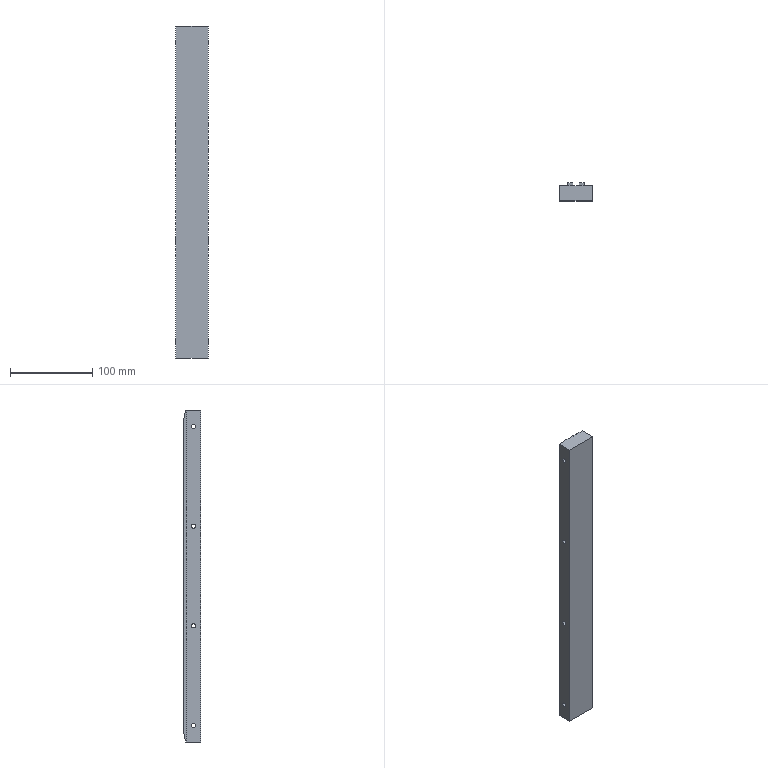Part | SolidWorks | features BaseBody 1 | 1 solid | 26 faces | box 40 x 21.5 x 403 mm | volume 303148 mm3 | plane 18 | cylinder 8 | commonest cylinder face diameters 5.2 x8
STEP:
#1=CARTESIAN_POINT('',(3866.757,551.261,63.1));
#2=VERTEX_POINT('',#1);
#3=CARTESIAN_POINT('',(3866.757,551.261,57.9));
#4=VERTEX_POINT('',#3);
#5=CARTESIAN_POINT('',(3866.757,551.261,60.5));
#6=DIRECTION('',(1.,0.,0.));
#7=DIRECTION('',(0.,0.,-1.));
#8=AXIS2_PLACEMENT_3D('',#5,#6,#7);
#9=CIRCLE('',#8,2.6);
#10=EDGE_CURVE('',#2,#4,#9,.T.);
#11=ORIENTED_EDGE('',*,*,#10,.F.);
#12=CARTESIAN_POINT('',(3906.757,551.261,63.1));
#13=VERTEX_POINT('',#12);
#14=CARTESIAN_POINT('',(3866.757,551.261,63.1));
#15=DIRECTION('',(1.,0.,0.));
#16=VECTOR('',#15,1000.);
#17=LINE('',#14,#16);
#18=EDGE_CURVE('',#2,#13,#17,.T.);
#19=ORIENTED_EDGE('',*,*,#18,.T.);
#20=CARTESIAN_POINT('',(3906.757,551.261,57.9));
#21=VERTEX_POINT('',#20);
#22=CARTESIAN_POINT('',(3906.757,551.261,60.5));
#23=DIRECTION('',(1.,0.,0.));
#24=DIRECTION('',(0.,0.,-1.));
#25=AXIS2_PLACEMENT_3D('',#22,#23,#24);
#26=CIRCLE('',#25,2.6);
#27=EDGE_CURVE('',#13,#21,#26,.T.);
#28=ORIENTED_EDGE('',*,*,#27,.T.);
#29=CARTESIAN_POINT('',(3866.757,551.261,57.9));
#30=DIRECTION('',(1.,0.,0.));
#31=VECTOR('',#30,1000.);
#32=LINE('',#29,#31);
#33=EDGE_CURVE('',#4,#21,#32,.T.);
#34=ORIENTED_EDGE('',*,*,#33,.F.);
#35=EDGE_LOOP('',(#11,#19,#28,#34));
#36=FACE_OUTER_BOUND('',#35,.T.);
#37=CARTESIAN_POINT('',(3866.757,551.261,60.5));
#38=DIRECTION('',(1.,0.,0.));
#39=DIRECTION('',(0.,0.,-1.));
#40=AXIS2_PLACEMENT_3D('',#37,#38,#39);
#41=CYLINDRICAL_SURFACE('',#40,2.6);
#42=ADVANCED_FACE('',(#36),#41,.F.);
#43=CARTESIAN_POINT('',(3866.757,551.261,184.1));
#44=VERTEX_POINT('',#43);
#45=CARTESIAN_POINT('',(3866.757,551.261,178.9));
#46=VERTEX_POINT('',#45);
#47=CARTESIAN_POINT('',(3866.757,551.261,181.5));
#48=DIRECTION('',(1.,0.,0.));
#49=DIRECTION('',(0.,0.,-1.));
#50=AXIS2_PLACEMENT_3D('',#47,#48,#49);
#51=CIRCLE('',#50,2.6);
#52=EDGE_CURVE('',#44,#46,#51,.T.);
#53=ORIENTED_EDGE('',*,*,#52,.F.);
#54=CARTESIAN_POINT('',(3906.757,551.261,184.1));
#55=VERTEX_POINT('',#54);
#56=CARTESIAN_POINT('',(3866.757,551.261,184.1));
#57=DIRECTION('',(1.,0.,0.));
#58=VECTOR('',#57,1000.);
#59=LINE('',#56,#58);
#60=EDGE_CURVE('',#44,#55,#59,.T.);
#61=ORIENTED_EDGE('',*,*,#60,.T.);
#62=CARTESIAN_POINT('',(3906.757,551.261,178.9));
#63=VERTEX_POINT('',#62);
#64=CARTESIAN_POINT('',(3906.757,551.261,181.5));
#65=DIRECTION('',(1.,0.,0.));
#66=DIRECTION('',(0.,0.,-1.));
#67=AXIS2_PLACEMENT_3D('',#64,#65,#66);
#68=CIRCLE('',#67,2.6);
#69=EDGE_CURVE('',#55,#63,#68,.T.);
#70=ORIENTED_EDGE('',*,*,#69,.T.);
#71=CARTESIAN_POINT('',(3866.757,551.261,178.9));
#72=DIRECTION('',(1.,0.,0.));
#73=VECTOR('',#72,1000.);
#74=LINE('',#71,#73);
#75=EDGE_CURVE('',#46,#63,#74,.T.);
#76=ORIENTED_EDGE('',*,*,#75,.F.);
#77=EDGE_LOOP('',(#53,#61,#70,#76));
#78=FACE_OUTER_BOUND('',#77,.T.);
#79=CARTESIAN_POINT('',(3866.757,551.261,181.5));
#80=DIRECTION('',(1.,0.,0.));
#81=DIRECTION('',(0.,0.,-1.));
#82=AXIS2_PLACEMENT_3D('',#79,#80,#81);
#83=CYLINDRICAL_SURFACE('',#82,2.6);
#84=ADVANCED_FACE('',(#78),#83,.F.);
#85=CARTESIAN_POINT('',(3866.757,551.261,-57.9));
#86=VERTEX_POINT('',#85);
#87=CARTESIAN_POINT('',(3866.757,551.261,-63.1));
#88=VERTEX_POINT('',#87);
#89=CARTESIAN_POINT('',(3866.757,551.261,-60.5));
#90=DIRECTION('',(1.,0.,0.));
#91=DIRECTION('',(0.,0.,-1.));
#92=AXIS2_PLACEMENT_3D('',#89,#90,#91);
#93=CIRCLE('',#92,2.6);
#94=EDGE_CURVE('',#86,#88,#93,.T.);
#95=ORIENTED_EDGE('',*,*,#94,.F.);
#96=CARTESIAN_POINT('',(3906.757,551.261,-57.9));
#97=VERTEX_POINT('',#96);
#98=CARTESIAN_POINT('',(3866.757,551.261,-57.9));
#99=DIRECTION('',(1.,0.,0.));
#100=VECTOR('',#99,1000.);
#101=LINE('',#98,#100);
#102=EDGE_CURVE('',#86,#97,#101,.T.);
#103=ORIENTED_EDGE('',*,*,#102,.T.);
#104=CARTESIAN_POINT('',(3906.757,551.261,-63.1));
#105=VERTEX_POINT('',#104);
#106=CARTESIAN_POINT('',(3906.757,551.261,-60.5));
#107=DIRECTION('',(1.,0.,0.));
#108=DIRECTION('',(0.,0.,-1.));
#109=AXIS2_PLACEMENT_3D('',#106,#107,#108);
#110=CIRCLE('',#109,2.6);
#111=EDGE_CURVE('',#97,#105,#110,.T.);
#112=ORIENTED_EDGE('',*,*,#111,.T.);
#113=CARTESIAN_POINT('',(3866.757,551.261,-63.1));
#114=DIRECTION('',(1.,0.,0.));
#115=VECTOR('',#114,1000.);
#116=LINE('',#113,#115);
#117=EDGE_CURVE('',#88,#105,#116,.T.);
#118=ORIENTED_EDGE('',*,*,#117,.F.);
#119=EDGE_LOOP('',(#95,#103,#112,#118));
#120=FACE_OUTER_BOUND('',#119,.T.);
#121=CARTESIAN_POINT('',(3866.757,551.261,-60.5));
#122=DIRECTION('',(1.,0.,0.));
#123=DIRECTION('',(0.,0.,-1.));
#124=AXIS2_PLACEMENT_3D('',#121,#122,#123);
#125=CYLINDRICAL_SURFACE('',#124,2.6);
#126=ADVANCED_FACE('',(#120),#125,.F.);
#127=CARTESIAN_POINT('',(3866.757,551.261,-178.9));
#128=VERTEX_POINT('',#127);
#129=CARTESIAN_POINT('',(3866.757,551.261,-184.1));
#130=VERTEX_POINT('',#129);
#131=CARTESIAN_POINT('',(3866.757,551.261,-181.5));
#132=DIRECTION('',(1.,0.,0.));
#133=DIRECTION('',(0.,0.,-1.));
#134=AXIS2_PLACEMENT_3D('',#131,#132,#133);
#135=CIRCLE('',#134,2.6);
#136=EDGE_CURVE('',#128,#130,#135,.T.);
#137=ORIENTED_EDGE('',*,*,#136,.F.);
#138=CARTESIAN_POINT('',(3906.757,551.261,-178.9));
#139=VERTEX_POINT('',#138);
#140=CARTESIAN_POINT('',(3866.757,551.261,-178.9));
#141=DIRECTION('',(1.,0.,0.));
#142=VECTOR('',#141,1000.);
#143=LINE('',#140,#142);
#144=EDGE_CURVE('',#128,#139,#143,.T.);
#145=ORIENTED_EDGE('',*,*,#144,.T.);
#146=CARTESIAN_POINT('',(3906.757,551.261,-184.1));
#147=VERTEX_POINT('',#146);
#148=CARTESIAN_POINT('',(3906.757,551.261,-181.5));
#149=DIRECTION('',(1.,0.,0.));
#150=DIRECTION('',(0.,0.,-1.));
#151=AXIS2_PLACEMENT_3D('',#148,#149,#150);
#152=CIRCLE('',#151,2.6);
#153=EDGE_CURVE('',#139,#147,#152,.T.);
#154=ORIENTED_EDGE('',*,*,#153,.T.);
#155=CARTESIAN_POINT('',(3866.757,551.261,-184.1));
#156=DIRECTION('',(1.,0.,0.));
#157=VECTOR('',#156,1000.);
#158=LINE('',#155,#157);
#159=EDGE_CURVE('',#130,#147,#158,.T.);
#160=ORIENTED_EDGE('',*,*,#159,.F.);
#161=EDGE_LOOP('',(#137,#145,#154,#160));
#162=FACE_OUTER_BOUND('',#161,.T.);
#163=CARTESIAN_POINT('',(3866.757,551.261,-181.5));
#164=DIRECTION('',(1.,0.,0.));
#165=DIRECTION('',(0.,0.,-1.));
#166=AXIS2_PLACEMENT_3D('',#163,#164,#165);
#167=CYLINDRICAL_SURFACE('',#166,2.6);
#168=ADVANCED_FACE('',(#162),#167,.F.);
#169=ORIENTED_EDGE('',*,*,#144,.F.);
#170=CARTESIAN_POINT('',(3866.757,551.261,-181.5));
#171=DIRECTION('',(1.,0.,0.));
#172=DIRECTION('',(0.,0.,-1.));
#173=AXIS2_PLACEMENT_3D('',#170,#171,#172);
#174=CIRCLE('',#173,2.6);
#175=EDGE_CURVE('',#130,#128,#174,.T.);
#176=ORIENTED_EDGE('',*,*,#175,.F.);
#177=ORIENTED_EDGE('',*,*,#159,.T.);
#178=CARTESIAN_POINT('',(3906.757,551.261,-181.5));
#179=DIRECTION('',(1.,0.,0.));
#180=DIRECTION('',(0.,0.,-1.));
#181=AXIS2_PLACEMENT_3D('',#178,#179,#180);
#182=CIRCLE('',#181,2.6);
#183=EDGE_CURVE('',#147,#139,#182,.T.);
#184=ORIENTED_EDGE('',*,*,#183,.T.);
#185=EDGE_LOOP('',(#169,#176,#177,#184));
#186=FACE_OUTER_BOUND('',#185,.T.);
#187=CARTESIAN_POINT('',(3866.757,551.261,-181.5));
#188=DIRECTION('',(1.,0.,0.));
#189=DIRECTION('',(0.,0.,-1.));
#190=AXIS2_PLACEMENT_3D('',#187,#188,#189);
#191=CYLINDRICAL_SURFACE('',#190,2.6);
#192=ADVANCED_FACE('',(#186),#191,.F.);
#193=ORIENTED_EDGE('',*,*,#102,.F.);
#194=CARTESIAN_POINT('',(3866.757,551.261,-60.5));
#195=DIRECTION('',(1.,0.,0.));
#196=DIRECTION('',(0.,0.,-1.));
#197=AXIS2_PLACEMENT_3D('',#194,#195,#196);
#198=CIRCLE('',#197,2.6);
#199=EDGE_CURVE('',#88,#86,#198,.T.);
#200=ORIENTED_EDGE('',*,*,#199,.F.);
#201=ORIENTED_EDGE('',*,*,#117,.T.);
#202=CARTESIAN_POINT('',(3906.757,551.261,-60.5));
#203=DIRECTION('',(1.,0.,0.));
#204=DIRECTION('',(0.,0.,-1.));
#205=AXIS2_PLACEMENT_3D('',#202,#203,#204);
#206=CIRCLE('',#205,2.6);
#207=EDGE_CURVE('',#105,#97,#206,.T.);
#208=ORIENTED_EDGE('',*,*,#207,.T.);
#209=EDGE_LOOP('',(#193,#200,#201,#208));
#210=FACE_OUTER_BOUND('',#209,.T.);
#211=CARTESIAN_POINT('',(3866.757,551.261,-60.5));
#212=DIRECTION('',(1.,0.,0.));
#213=DIRECTION('',(0.,0.,-1.));
#214=AXIS2_PLACEMENT_3D('',#211,#212,#213);
#215=CYLINDRICAL_SURFACE('',#214,2.6);
#216=ADVANCED_FACE('',(#210),#215,.F.);
#217=CARTESIAN_POINT('',(3896.757,560.261,-201.5));
#218=VERTEX_POINT('',#217);
#219=CARTESIAN_POINT('',(3896.757,560.761,-201.5));
#220=VERTEX_POINT('',#219);
#221=CARTESIAN_POINT('',(3896.757,560.261,-201.5));
#222=DIRECTION('',(0.,1.,0.));
#223=VECTOR('',#222,1000.);
#224=LINE('',#221,#223);
#225=EDGE_CURVE('',#218,#220,#224,.T.);
#226=ORIENTED_EDGE('',*,*,#225,.T.);
#227=CARTESIAN_POINT('',(3896.757,563.761,-186.5));
#228=VERTEX_POINT('',#227);
#229=CARTESIAN_POINT('',(3896.757,563.761,-186.5));
#230=DIRECTION('',(0.,0.1961,0.9806));
#231=VECTOR('',#230,1000.);
#232=LINE('',#229,#231);
#233=EDGE_CURVE('',#220,#228,#232,.T.);
#234=ORIENTED_EDGE('',*,*,#233,.T.);
#235=CARTESIAN_POINT('',(3896.757,563.761,186.5));
#236=VERTEX_POINT('',#235);
#237=CARTESIAN_POINT('',(3896.757,563.761,201.5));
#238=DIRECTION('',(0.,0.,-1.));
#239=VECTOR('',#238,1000.);
#240=LINE('',#237,#239);
#241=EDGE_CURVE('',#236,#228,#240,.T.);
#242=ORIENTED_EDGE('',*,*,#241,.F.);
#243=CARTESIAN_POINT('',(3896.757,560.761,201.5));
#244=VERTEX_POINT('',#243);
#245=CARTESIAN_POINT('',(3896.757,560.761,201.5));
#246=DIRECTION('',(0.,-0.1961,0.9806));
#247=VECTOR('',#246,1000.);
#248=LINE('',#245,#247);
#249=EDGE_CURVE('',#236,#244,#248,.T.);
#250=ORIENTED_EDGE('',*,*,#249,.T.);
#251=CARTESIAN_POINT('',(3896.757,560.261,201.5));
#252=VERTEX_POINT('',#251);
#253=CARTESIAN_POINT('',(3896.757,560.261,201.5));
#254=DIRECTION('',(0.,1.,0.));
#255=VECTOR('',#254,1000.);
#256=LINE('',#253,#255);
#257=EDGE_CURVE('',#252,#244,#256,.T.);
#258=ORIENTED_EDGE('',*,*,#257,.F.);
#259=CARTESIAN_POINT('',(3896.757,560.261,201.5));
#260=DIRECTION('',(0.,0.,-1.));
#261=VECTOR('',#260,1000.);
#262=LINE('',#259,#261);
#263=EDGE_CURVE('',#252,#218,#262,.T.);
#264=ORIENTED_EDGE('',*,*,#263,.T.);
#265=EDGE_LOOP('',(#226,#234,#242,#250,#258,#264));
#266=FACE_OUTER_BOUND('',#265,.T.);
#267=CARTESIAN_POINT('',(3896.757,560.261,201.5));
#268=DIRECTION('',(-1.,0.,0.));
#269=DIRECTION('',(0.,0.,1.));
#270=AXIS2_PLACEMENT_3D('',#267,#268,#269);
#271=PLANE('',#270);
#272=ADVANCED_FACE('',(#266),#271,.F.);
#273=ORIENTED_EDGE('',*,*,#241,.T.);
#274=CARTESIAN_POINT('',(3890.757,563.761,-186.5));
#275=VERTEX_POINT('',#274);
#276=CARTESIAN_POINT('',(3896.757,563.761,-186.5));
#277=DIRECTION('',(-1.,0.,0.));
#278=VECTOR('',#277,1000.);
#279=LINE('',#276,#278);
#280=EDGE_CURVE('',#228,#275,#279,.T.);
#281=ORIENTED_EDGE('',*,*,#280,.T.);
#282=CARTESIAN_POINT('',(3890.757,563.761,186.5));
#283=VERTEX_POINT('',#282);
#284=CARTESIAN_POINT('',(3890.757,563.761,201.5));
#285=DIRECTION('',(0.,0.,-1.));
#286=VECTOR('',#285,1000.);
#287=LINE('',#284,#286);
#288=EDGE_CURVE('',#283,#275,#287,.T.);
#289=ORIENTED_EDGE('',*,*,#288,.F.);
#290=CARTESIAN_POINT('',(3896.757,563.761,186.5));
#291=DIRECTION('',(1.,0.,0.));
#292=VECTOR('',#291,1000.);
#293=LINE('',#290,#292);
#294=EDGE_CURVE('',#283,#236,#293,.T.);
#295=ORIENTED_EDGE('',*,*,#294,.T.);
#296=EDGE_LOOP('',(#273,#281,#289,#295));
#297=FACE_OUTER_BOUND('',#296,.T.);
#298=CARTESIAN_POINT('',(3896.757,563.761,201.5));
#299=DIRECTION('',(0.,-1.,0.));
#300=DIRECTION('',(0.,0.,-1.));
#301=AXIS2_PLACEMENT_3D('',#298,#299,#300);
#302=PLANE('',#301);
#303=ADVANCED_FACE('',(#297),#302,.F.);
#304=ORIENTED_EDGE('',*,*,#288,.T.);
#305=CARTESIAN_POINT('',(3890.757,560.761,-201.5));
#306=VERTEX_POINT('',#305);
#307=CARTESIAN_POINT('',(3890.757,563.761,-186.5));
#308=DIRECTION('',(0.,-0.1961,-0.9806));
#309=VECTOR('',#308,1000.);
#310=LINE('',#307,#309);
#311=EDGE_CURVE('',#275,#306,#310,.T.);
#312=ORIENTED_EDGE('',*,*,#311,.T.);
#313=CARTESIAN_POINT('',(3890.757,560.261,-201.5));
#314=VERTEX_POINT('',#313);
#315=CARTESIAN_POINT('',(3890.757,563.761,-201.5));
#316=DIRECTION('',(0.,-1.,0.));
#317=VECTOR('',#316,1000.);
#318=LINE('',#315,#317);
#319=EDGE_CURVE('',#306,#314,#318,.T.);
#320=ORIENTED_EDGE('',*,*,#319,.T.);
#321=CARTESIAN_POINT('',(3890.757,560.261,201.5));
#322=VERTEX_POINT('',#321);
#323=CARTESIAN_POINT('',(3890.757,560.261,201.5));
#324=DIRECTION('',(0.,0.,-1.));
#325=VECTOR('',#324,1000.);
#326=LINE('',#323,#325);
#327=EDGE_CURVE('',#322,#314,#326,.T.);
#328=ORIENTED_EDGE('',*,*,#327,.F.);
#329=CARTESIAN_POINT('',(3890.757,560.761,201.5));
#330=VERTEX_POINT('',#329);
#331=CARTESIAN_POINT('',(3890.757,563.761,201.5));
#332=DIRECTION('',(0.,-1.,0.));
#333=VECTOR('',#332,1000.);
#334=LINE('',#331,#333);
#335=EDGE_CURVE('',#330,#322,#334,.T.);
#336=ORIENTED_EDGE('',*,*,#335,.F.);
#337=CARTESIAN_POINT('',(3890.757,560.761,201.5));
#338=DIRECTION('',(0.,0.1961,-0.9806));
#339=VECTOR('',#338,1000.);
#340=LINE('',#337,#339);
#341=EDGE_CURVE('',#330,#283,#340,.T.);
#342=ORIENTED_EDGE('',*,*,#341,.T.);
#343=EDGE_LOOP('',(#304,#312,#320,#328,#336,#342));
#344=FACE_OUTER_BOUND('',#343,.T.);
#345=CARTESIAN_POINT('',(3890.757,563.761,201.5));
#346=DIRECTION('',(1.,0.,0.));
#347=DIRECTION('',(0.,0.,-1.));
#348=AXIS2_PLACEMENT_3D('',#345,#346,#347);
#349=PLANE('',#348);
#350=ADVANCED_FACE('',(#344),#349,.F.);
#351=CARTESIAN_POINT('',(3882.757,560.261,-201.5));
#352=VERTEX_POINT('',#351);
#353=CARTESIAN_POINT('',(3882.757,560.261,-201.5));
#354=DIRECTION('',(-1.,0.,0.));
#355=VECTOR('',#354,1000.);
#356=LINE('',#353,#355);
#357=EDGE_CURVE('',#314,#352,#356,.T.);
#358=ORIENTED_EDGE('',*,*,#357,.T.);
#359=CARTESIAN_POINT('',(3882.757,560.261,201.5));
#360=VERTEX_POINT('',#359);
#361=CARTESIAN_POINT('',(3882.757,560.261,201.5));
#362=DIRECTION('',(0.,0.,-1.));
#363=VECTOR('',#362,1000.);
#364=LINE('',#361,#363);
#365=EDGE_CURVE('',#360,#352,#364,.T.);
#366=ORIENTED_EDGE('',*,*,#365,.F.);
#367=CARTESIAN_POINT('',(3882.757,560.261,201.5));
#368=DIRECTION('',(-1.,0.,0.));
#369=VECTOR('',#368,1000.);
#370=LINE('',#367,#369);
#371=EDGE_CURVE('',#322,#360,#370,.T.);
#372=ORIENTED_EDGE('',*,*,#371,.F.);
#373=ORIENTED_EDGE('',*,*,#327,.T.);
#374=EDGE_LOOP('',(#358,#366,#372,#373));
#375=FACE_OUTER_BOUND('',#374,.T.);
#376=CARTESIAN_POINT('',(3882.757,560.261,201.5));
#377=DIRECTION('',(0.,-1.,0.));
#378=DIRECTION('',(0.,0.,-1.));
#379=AXIS2_PLACEMENT_3D('',#376,#377,#378);
#380=PLANE('',#379);
#381=ADVANCED_FACE('',(#375),#380,.F.);
#382=CARTESIAN_POINT('',(3882.757,560.761,-201.5));
#383=VERTEX_POINT('',#382);
#384=CARTESIAN_POINT('',(3882.757,560.261,-201.5));
#385=DIRECTION('',(0.,1.,0.));
#386=VECTOR('',#385,1000.);
#387=LINE('',#384,#386);
#388=EDGE_CURVE('',#352,#383,#387,.T.);
#389=ORIENTED_EDGE('',*,*,#388,.T.);
#390=CARTESIAN_POINT('',(3882.757,563.761,-186.5));
#391=VERTEX_POINT('',#390);
#392=CARTESIAN_POINT('',(3882.757,563.761,-186.5));
#393=DIRECTION('',(0.,0.1961,0.9806));
#394=VECTOR('',#393,1000.);
#395=LINE('',#392,#394);
#396=EDGE_CURVE('',#383,#391,#395,.T.);
#397=ORIENTED_EDGE('',*,*,#396,.T.);
#398=CARTESIAN_POINT('',(3882.757,563.761,186.5));
#399=VERTEX_POINT('',#398);
#400=CARTESIAN_POINT('',(3882.757,563.761,201.5));
#401=DIRECTION('',(0.,0.,-1.));
#402=VECTOR('',#401,1000.);
#403=LINE('',#400,#402);
#404=EDGE_CURVE('',#399,#391,#403,.T.);
#405=ORIENTED_EDGE('',*,*,#404,.F.);
#406=CARTESIAN_POINT('',(3882.757,560.761,201.5));
#407=VERTEX_POINT('',#406);
#408=CARTESIAN_POINT('',(3882.757,560.761,201.5));
#409=DIRECTION('',(0.,-0.1961,0.9806));
#410=VECTOR('',#409,1000.);
#411=LINE('',#408,#410);
#412=EDGE_CURVE('',#399,#407,#411,.T.);
#413=ORIENTED_EDGE('',*,*,#412,.T.);
#414=CARTESIAN_POINT('',(3882.757,560.261,201.5));
#415=DIRECTION('',(0.,1.,0.));
#416=VECTOR('',#415,1000.);
#417=LINE('',#414,#416);
#418=EDGE_CURVE('',#360,#407,#417,.T.);
#419=ORIENTED_EDGE('',*,*,#418,.F.);
#420=ORIENTED_EDGE('',*,*,#365,.T.);
#421=EDGE_LOOP('',(#389,#397,#405,#413,#419,#420));
#422=FACE_OUTER_BOUND('',#421,.T.);
#423=CARTESIAN_POINT('',(3882.757,560.261,201.5));
#424=DIRECTION('',(-1.,0.,0.));
#425=DIRECTION('',(0.,0.,1.));
#426=AXIS2_PLACEMENT_3D('',#423,#424,#425);
#427=PLANE('',#426);
#428=ADVANCED_FACE('',(#422),#427,.F.);
#429=ORIENTED_EDGE('',*,*,#404,.T.);
#430=CARTESIAN_POINT('',(3876.757,563.761,-186.5));
#431=VERTEX_POINT('',#430);
#432=CARTESIAN_POINT('',(3882.757,563.761,-186.5));
#433=DIRECTION('',(-1.,0.,0.));
#434=VECTOR('',#433,1000.);
#435=LINE('',#432,#434);
#436=EDGE_CURVE('',#391,#431,#435,.T.);
#437=ORIENTED_EDGE('',*,*,#436,.T.);
#438=CARTESIAN_POINT('',(3876.757,563.761,186.5));
#439=VERTEX_POINT('',#438);
#440=CARTESIAN_POINT('',(3876.757,563.761,201.5));
#441=DIRECTION('',(0.,0.,-1.));
#442=VECTOR('',#441,1000.);
#443=LINE('',#440,#442);
#444=EDGE_CURVE('',#439,#431,#443,.T.);
#445=ORIENTED_EDGE('',*,*,#444,.F.);
#446=CARTESIAN_POINT('',(3882.757,563.761,186.5));
#447=DIRECTION('',(1.,0.,0.));
#448=VECTOR('',#447,1000.);
#449=LINE('',#446,#448);
#450=EDGE_CURVE('',#439,#399,#449,.T.);
#451=ORIENTED_EDGE('',*,*,#450,.T.);
#452=EDGE_LOOP('',(#429,#437,#445,#451));
#453=FACE_OUTER_BOUND('',#452,.T.);
#454=CARTESIAN_POINT('',(3882.757,563.761,201.5));
#455=DIRECTION('',(0.,-1.,0.));
#456=DIRECTION('',(0.,0.,-1.));
#457=AXIS2_PLACEMENT_3D('',#454,#455,#456);
#458=PLANE('',#457);
#459=ADVANCED_FACE('',(#453),#458,.F.);
#460=ORIENTED_EDGE('',*,*,#444,.T.);
#461=CARTESIAN_POINT('',(3876.757,560.761,-201.5));
#462=VERTEX_POINT('',#461);
#463=CARTESIAN_POINT('',(3876.757,563.761,-186.5));
#464=DIRECTION('',(0.,-0.1961,-0.9806));
#465=VECTOR('',#464,1000.);
#466=LINE('',#463,#465);
#467=EDGE_CURVE('',#431,#462,#466,.T.);
#468=ORIENTED_EDGE('',*,*,#467,.T.);
#469=CARTESIAN_POINT('',(3876.757,560.261,-201.5));
#470=VERTEX_POINT('',#469);
#471=CARTESIAN_POINT('',(3876.757,563.761,-201.5));
#472=DIRECTION('',(0.,-1.,0.));
#473=VECTOR('',#472,1000.);
#474=LINE('',#471,#473);
#475=EDGE_CURVE('',#462,#470,#474,.T.);
#476=ORIENTED_EDGE('',*,*,#475,.T.);
#477=CARTESIAN_POINT('',(3876.757,560.261,201.5));
#478=VERTEX_POINT('',#477);
#479=CARTESIAN_POINT('',(3876.757,560.261,201.5));
#480=DIRECTION('',(0.,0.,-1.));
#481=VECTOR('',#480,1000.);
#482=LINE('',#479,#481);
#483=EDGE_CURVE('',#478,#470,#482,.T.);
#484=ORIENTED_EDGE('',*,*,#483,.F.);
#485=CARTESIAN_POINT('',(3876.757,560.761,201.5));
#486=VERTEX_POINT('',#485);
#487=CARTESIAN_POINT('',(3876.757,563.761,201.5));
#488=DIRECTION('',(0.,-1.,0.));
#489=VECTOR('',#488,1000.);
#490=LINE('',#487,#489);
#491=EDGE_CURVE('',#486,#478,#490,.T.);
#492=ORIENTED_EDGE('',*,*,#491,.F.);
#493=CARTESIAN_POINT('',(3876.757,560.761,201.5));
#494=DIRECTION('',(0.,0.1961,-0.9806));
#495=VECTOR('',#494,1000.);
#496=LINE('',#493,#495);
#497=EDGE_CURVE('',#486,#439,#496,.T.);
#498=ORIENTED_EDGE('',*,*,#497,.T.);
#499=EDGE_LOOP('',(#460,#468,#476,#484,#492,#498));
#500=FACE_OUTER_BOUND('',#499,.T.);
#501=CARTESIAN_POINT('',(3876.757,563.761,201.5));
#502=DIRECTION('',(1.,0.,0.));
#503=DIRECTION('',(0.,0.,-1.));
#504=AXIS2_PLACEMENT_3D('',#501,#502,#503);
#505=PLANE('',#504);
#506=ADVANCED_FACE('',(#500),#505,.F.);
#507=CARTESIAN_POINT('',(3866.757,560.261,-201.5));
#508=VERTEX_POINT('',#507);
#509=CARTESIAN_POINT('',(3866.757,560.261,-201.5));
#510=DIRECTION('',(-1.,0.,0.));
#511=VECTOR('',#510,1000.);
#512=LINE('',#509,#511);
#513=EDGE_CURVE('',#470,#508,#512,.T.);
#514=ORIENTED_EDGE('',*,*,#513,.T.);
#515=CARTESIAN_POINT('',(3866.757,560.261,201.5));
#516=VERTEX_POINT('',#515);
#517=CARTESIAN_POINT('',(3866.757,560.261,201.5));
#518=DIRECTION('',(0.,0.,-1.));
#519=VECTOR('',#518,1000.);
#520=LINE('',#517,#519);
#521=EDGE_CURVE('',#516,#508,#520,.T.);
#522=ORIENTED_EDGE('',*,*,#521,.F.);
#523=CARTESIAN_POINT('',(3866.757,560.261,201.5));
#524=DIRECTION('',(-1.,0.,0.));
#525=VECTOR('',#524,1000.);
#526=LINE('',#523,#525);
#527=EDGE_CURVE('',#478,#516,#526,.T.);
#528=ORIENTED_EDGE('',*,*,#527,.F.);
#529=ORIENTED_EDGE('',*,*,#483,.T.);
#530=EDGE_LOOP('',(#514,#522,#528,#529));
#531=FACE_OUTER_BOUND('',#530,.T.);
#532=CARTESIAN_POINT('',(3866.757,560.261,201.5));
#533=DIRECTION('',(0.,-1.,0.));
#534=DIRECTION('',(0.,0.,-1.));
#535=AXIS2_PLACEMENT_3D('',#532,#533,#534);
#536=PLANE('',#535);
#537=ADVANCED_FACE('',(#531),#536,.F.);
#538=CARTESIAN_POINT('',(3866.757,551.261,60.5));
#539=DIRECTION('',(1.,0.,0.));
#540=DIRECTION('',(0.,0.,-1.));
#541=AXIS2_PLACEMENT_3D('',#538,#539,#540);
#542=CIRCLE('',#541,2.6);
#543=EDGE_CURVE('',#4,#2,#542,.T.);
#544=ORIENTED_EDGE('',*,*,#543,.T.);
#545=ORIENTED_EDGE('',*,*,#10,.T.);
#546=EDGE_LOOP('',(#544,#545));
#547=FACE_BOUND('',#546,.T.);
#548=CARTESIAN_POINT('',(3866.757,551.261,181.5));
#549=DIRECTION('',(1.,0.,0.));
#550=DIRECTION('',(0.,0.,-1.));
#551=AXIS2_PLACEMENT_3D('',#548,#549,#550);
#552=CIRCLE('',#551,2.6);
#553=EDGE_CURVE('',#46,#44,#552,.T.);
#554=ORIENTED_EDGE('',*,*,#553,.T.);
#555=ORIENTED_EDGE('',*,*,#52,.T.);
#556=EDGE_LOOP('',(#554,#555));
#557=FACE_BOUND('',#556,.T.);
#558=CARTESIAN_POINT('',(3866.757,542.261,-201.5));
#559=VERTEX_POINT('',#558);
#560=CARTESIAN_POINT('',(3866.757,542.261,-201.5));
#561=DIRECTION('',(0.,-1.,0.));
#562=VECTOR('',#561,1000.);
#563=LINE('',#560,#562);
#564=EDGE_CURVE('',#508,#559,#563,.T.);
#565=ORIENTED_EDGE('',*,*,#564,.T.);
#566=CARTESIAN_POINT('',(3866.757,542.261,201.5));
#567=VERTEX_POINT('',#566);
#568=CARTESIAN_POINT('',(3866.757,542.261,201.5));
#569=DIRECTION('',(0.,0.,-1.));
#570=VECTOR('',#569,1000.);
#571=LINE('',#568,#570);
#572=EDGE_CURVE('',#567,#559,#571,.T.);
#573=ORIENTED_EDGE('',*,*,#572,.F.);
#574=CARTESIAN_POINT('',(3866.757,542.261,201.5));
#575=DIRECTION('',(0.,-1.,0.));
#576=VECTOR('',#575,1000.);
#577=LINE('',#574,#576);
#578=EDGE_CURVE('',#516,#567,#577,.T.);
#579=ORIENTED_EDGE('',*,*,#578,.F.);
#580=ORIENTED_EDGE('',*,*,#521,.T.);
#581=EDGE_LOOP('',(#565,#573,#579,#580));
#582=FACE_OUTER_BOUND('',#581,.T.);
#583=ORIENTED_EDGE('',*,*,#199,.T.);
#584=ORIENTED_EDGE('',*,*,#94,.T.);
#585=EDGE_LOOP('',(#583,#584));
#586=FACE_BOUND('',#585,.T.);
#587=ORIENTED_EDGE('',*,*,#175,.T.);
#588=ORIENTED_EDGE('',*,*,#136,.T.);
#589=EDGE_LOOP('',(#587,#588));
#590=FACE_BOUND('',#589,.T.);
#591=CARTESIAN_POINT('',(3866.757,542.261,201.5));
#592=DIRECTION('',(1.,0.,0.));
#593=DIRECTION('',(0.,0.,-1.));
#594=AXIS2_PLACEMENT_3D('',#591,#592,#593);
#595=PLANE('',#594);
#596=ADVANCED_FACE('',(#547,#557,#582,#586,#590),#595,.F.);
#597=CARTESIAN_POINT('',(3906.757,542.261,-201.5));
#598=VERTEX_POINT('',#597);
#599=CARTESIAN_POINT('',(3906.757,542.261,-201.5));
#600=DIRECTION('',(1.,0.,0.));
#601=VECTOR('',#600,1000.);
#602=LINE('',#599,#601);
#603=EDGE_CURVE('',#559,#598,#602,.T.);
#604=ORIENTED_EDGE('',*,*,#603,.T.);
#605=CARTESIAN_POINT('',(3906.757,542.261,201.5));
#606=VERTEX_POINT('',#605);
#607=CARTESIAN_POINT('',(3906.757,542.261,201.5));
#608=DIRECTION('',(0.,0.,-1.));
#609=VECTOR('',#608,1000.);
#610=LINE('',#607,#609);
#611=EDGE_CURVE('',#606,#598,#610,.T.);
#612=ORIENTED_EDGE('',*,*,#611,.F.);
#613=CARTESIAN_POINT('',(3906.757,542.261,201.5));
#614=DIRECTION('',(1.,0.,0.));
#615=VECTOR('',#614,1000.);
#616=LINE('',#613,#615);
#617=EDGE_CURVE('',#567,#606,#616,.T.);
#618=ORIENTED_EDGE('',*,*,#617,.F.);
#619=ORIENTED_EDGE('',*,*,#572,.T.);
#620=EDGE_LOOP('',(#604,#612,#618,#619));
#621=FACE_OUTER_BOUND('',#620,.T.);
#622=CARTESIAN_POINT('',(3906.757,542.261,201.5));
#623=DIRECTION('',(0.,1.,0.));
#624=DIRECTION('',(0.,0.,1.));
#625=AXIS2_PLACEMENT_3D('',#622,#623,#624);
#626=PLANE('',#625);
#627=ADVANCED_FACE('',(#621),#626,.F.);
#628=CARTESIAN_POINT('',(3906.757,551.261,60.5));
#629=DIRECTION('',(1.,0.,0.));
#630=DIRECTION('',(0.,0.,-1.));
#631=AXIS2_PLACEMENT_3D('',#628,#629,#630);
#632=CIRCLE('',#631,2.6);
#633=EDGE_CURVE('',#21,#13,#632,.T.);
#634=ORIENTED_EDGE('',*,*,#633,.F.);
#635=ORIENTED_EDGE('',*,*,#27,.F.);
#636=EDGE_LOOP('',(#634,#635));
#637=FACE_BOUND('',#636,.T.);
#638=CARTESIAN_POINT('',(3906.757,551.261,181.5));
#639=DIRECTION('',(1.,0.,0.));
#640=DIRECTION('',(0.,0.,-1.));
#641=AXIS2_PLACEMENT_3D('',#638,#639,#640);
#642=CIRCLE('',#641,2.6);
#643=EDGE_CURVE('',#63,#55,#642,.T.);
#644=ORIENTED_EDGE('',*,*,#643,.F.);
#645=ORIENTED_EDGE('',*,*,#69,.F.);
#646=EDGE_LOOP('',(#644,#645));
#647=FACE_BOUND('',#646,.T.);
#648=CARTESIAN_POINT('',(3906.757,560.261,-201.5));
#649=VERTEX_POINT('',#648);
#650=CARTESIAN_POINT('',(3906.757,560.261,-201.5));
#651=DIRECTION('',(0.,1.,0.));
#652=VECTOR('',#651,1000.);
#653=LINE('',#650,#652);
#654=EDGE_CURVE('',#598,#649,#653,.T.);
#655=ORIENTED_EDGE('',*,*,#654,.T.);
#656=CARTESIAN_POINT('',(3906.757,560.261,201.5));
#657=VERTEX_POINT('',#656);
#658=CARTESIAN_POINT('',(3906.757,560.261,201.5));
#659=DIRECTION('',(0.,0.,-1.));
#660=VECTOR('',#659,1000.);
#661=LINE('',#658,#660);
#662=EDGE_CURVE('',#657,#649,#661,.T.);
#663=ORIENTED_EDGE('',*,*,#662,.F.);
#664=CARTESIAN_POINT('',(3906.757,560.261,201.5));
#665=DIRECTION('',(0.,1.,0.));
#666=VECTOR('',#665,1000.);
#667=LINE('',#664,#666);
#668=EDGE_CURVE('',#606,#657,#667,.T.);
#669=ORIENTED_EDGE('',*,*,#668,.F.);
#670=ORIENTED_EDGE('',*,*,#611,.T.);
#671=EDGE_LOOP('',(#655,#663,#669,#670));
#672=FACE_OUTER_BOUND('',#671,.T.);
#673=ORIENTED_EDGE('',*,*,#207,.F.);
#674=ORIENTED_EDGE('',*,*,#111,.F.);
#675=EDGE_LOOP('',(#673,#674));
#676=FACE_BOUND('',#675,.T.);
#677=ORIENTED_EDGE('',*,*,#183,.F.);
#678=ORIENTED_EDGE('',*,*,#153,.F.);
#679=EDGE_LOOP('',(#677,#678));
#680=FACE_BOUND('',#679,.T.);
#681=CARTESIAN_POINT('',(3906.757,560.261,201.5));
#682=DIRECTION('',(-1.,0.,0.));
#683=DIRECTION('',(0.,0.,1.));
#684=AXIS2_PLACEMENT_3D('',#681,#682,#683);
#685=PLANE('',#684);
#686=ADVANCED_FACE('',(#637,#647,#672,#676,#680),#685,.F.);
#687=CARTESIAN_POINT('',(3896.757,560.261,-201.5));
#688=DIRECTION('',(-1.,0.,0.));
#689=VECTOR('',#688,1000.);
#690=LINE('',#687,#689);
#691=EDGE_CURVE('',#649,#218,#690,.T.);
#692=ORIENTED_EDGE('',*,*,#691,.T.);
#693=ORIENTED_EDGE('',*,*,#263,.F.);
#694=CARTESIAN_POINT('',(3896.757,560.261,201.5));
#695=DIRECTION('',(-1.,0.,0.));
#696=VECTOR('',#695,1000.);
#697=LINE('',#694,#696);
#698=EDGE_CURVE('',#657,#252,#697,.T.);
#699=ORIENTED_EDGE('',*,*,#698,.F.);
#700=ORIENTED_EDGE('',*,*,#662,.T.);
#701=EDGE_LOOP('',(#692,#693,#699,#700));
#702=FACE_OUTER_BOUND('',#701,.T.);
#703=CARTESIAN_POINT('',(3896.757,560.261,201.5));
#704=DIRECTION('',(0.,-1.,0.));
#705=DIRECTION('',(0.,0.,-1.));
#706=AXIS2_PLACEMENT_3D('',#703,#704,#705);
#707=PLANE('',#706);
#708=ADVANCED_FACE('',(#702),#707,.F.);
#709=ORIENTED_EDGE('',*,*,#418,.T.);
#710=CARTESIAN_POINT('',(3876.757,560.761,201.5));
#711=DIRECTION('',(-1.,0.,0.));
#712=VECTOR('',#711,1000.);
#713=LINE('',#710,#712);
#714=EDGE_CURVE('',#407,#486,#713,.T.);
#715=ORIENTED_EDGE('',*,*,#714,.T.);
#716=ORIENTED_EDGE('',*,*,#491,.T.);
#717=ORIENTED_EDGE('',*,*,#527,.T.);
#718=ORIENTED_EDGE('',*,*,#578,.T.);
#719=ORIENTED_EDGE('',*,*,#617,.T.);
#720=ORIENTED_EDGE('',*,*,#668,.T.);
#721=ORIENTED_EDGE('',*,*,#698,.T.);
#722=ORIENTED_EDGE('',*,*,#257,.T.);
#723=CARTESIAN_POINT('',(3890.757,560.761,201.5));
#724=DIRECTION('',(-1.,0.,0.));
#725=VECTOR('',#724,1000.);
#726=LINE('',#723,#725);
#727=EDGE_CURVE('',#244,#330,#726,.T.);
#728=ORIENTED_EDGE('',*,*,#727,.T.);
#729=ORIENTED_EDGE('',*,*,#335,.T.);
#730=ORIENTED_EDGE('',*,*,#371,.T.);
#731=EDGE_LOOP('',(#709,#715,#716,#717,#718,#719,#720,#721,#722,#728,#729,#730));
#732=FACE_OUTER_BOUND('',#731,.T.);
#733=CARTESIAN_POINT('',(0.,0.,201.5));
#734=DIRECTION('',(0.,0.,1.));
#735=DIRECTION('',(1.,0.,0.));
#736=AXIS2_PLACEMENT_3D('',#733,#734,#735);
#737=PLANE('',#736);
#738=ADVANCED_FACE('',(#732),#737,.T.);
#739=ORIENTED_EDGE('',*,*,#475,.F.);
#740=CARTESIAN_POINT('',(0.,560.761,-201.5));
#741=DIRECTION('',(1.,0.,0.));
#742=VECTOR('',#741,1000.);
#743=LINE('',#740,#742);
#744=EDGE_CURVE('',#462,#383,#743,.T.);
#745=ORIENTED_EDGE('',*,*,#744,.T.);
#746=ORIENTED_EDGE('',*,*,#388,.F.);
#747=ORIENTED_EDGE('',*,*,#357,.F.);
#748=ORIENTED_EDGE('',*,*,#319,.F.);
#749=CARTESIAN_POINT('',(0.,560.761,-201.5));
#750=DIRECTION('',(1.,0.,0.));
#751=VECTOR('',#750,1000.);
#752=LINE('',#749,#751);
#753=EDGE_CURVE('',#306,#220,#752,.T.);
#754=ORIENTED_EDGE('',*,*,#753,.T.);
#755=ORIENTED_EDGE('',*,*,#225,.F.);
#756=ORIENTED_EDGE('',*,*,#691,.F.);
#757=ORIENTED_EDGE('',*,*,#654,.F.);
#758=ORIENTED_EDGE('',*,*,#603,.F.);
#759=ORIENTED_EDGE('',*,*,#564,.F.);
#760=ORIENTED_EDGE('',*,*,#513,.F.);
#761=EDGE_LOOP('',(#739,#745,#746,#747,#748,#754,#755,#756,#757,#758,#759,#760));
#762=FACE_OUTER_BOUND('',#761,.T.);
#763=CARTESIAN_POINT('',(0.,0.,-201.5));
#764=DIRECTION('',(0.,0.,1.));
#765=DIRECTION('',(1.,0.,0.));
#766=AXIS2_PLACEMENT_3D('',#763,#764,#765);
#767=PLANE('',#766);
#768=ADVANCED_FACE('',(#762),#767,.F.);
#769=ORIENTED_EDGE('',*,*,#412,.F.);
#770=ORIENTED_EDGE('',*,*,#450,.F.);
#771=ORIENTED_EDGE('',*,*,#497,.F.);
#772=ORIENTED_EDGE('',*,*,#714,.F.);
#773=EDGE_LOOP('',(#769,#770,#771,#772));
#774=FACE_OUTER_BOUND('',#773,.T.);
#775=CARTESIAN_POINT('',(0.,560.761,201.5));
#776=DIRECTION('',(0.,0.9806,0.1961));
#777=DIRECTION('',(1.,0.,0.));
#778=AXIS2_PLACEMENT_3D('',#775,#776,#777);
#779=PLANE('',#778);
#780=ADVANCED_FACE('',(#774),#779,.T.);
#781=ORIENTED_EDGE('',*,*,#249,.F.);
#782=ORIENTED_EDGE('',*,*,#294,.F.);
#783=ORIENTED_EDGE('',*,*,#341,.F.);
#784=ORIENTED_EDGE('',*,*,#727,.F.);
#785=EDGE_LOOP('',(#781,#782,#783,#784));
#786=FACE_OUTER_BOUND('',#785,.T.);
#787=CARTESIAN_POINT('',(0.,560.761,201.5));
#788=DIRECTION('',(0.,0.9806,0.1961));
#789=DIRECTION('',(1.,0.,0.));
#790=AXIS2_PLACEMENT_3D('',#787,#788,#789);
#791=PLANE('',#790);
#792=ADVANCED_FACE('',(#786),#791,.T.);
#793=ORIENTED_EDGE('',*,*,#396,.F.);
#794=ORIENTED_EDGE('',*,*,#744,.F.);
#795=ORIENTED_EDGE('',*,*,#467,.F.);
#796=ORIENTED_EDGE('',*,*,#436,.F.);
#797=EDGE_LOOP('',(#793,#794,#795,#796));
#798=FACE_OUTER_BOUND('',#797,.T.);
#799=CARTESIAN_POINT('',(3882.757,563.761,-186.5));
#800=DIRECTION('',(0.,-0.9806,0.1961));
#801=DIRECTION('',(-1.,0.,0.));
#802=AXIS2_PLACEMENT_3D('',#799,#800,#801);
#803=PLANE('',#802);
#804=ADVANCED_FACE('',(#798),#803,.F.);
#805=ORIENTED_EDGE('',*,*,#233,.F.);
#806=ORIENTED_EDGE('',*,*,#753,.F.);
#807=ORIENTED_EDGE('',*,*,#311,.F.);
#808=ORIENTED_EDGE('',*,*,#280,.F.);
#809=EDGE_LOOP('',(#805,#806,#807,#808));
#810=FACE_OUTER_BOUND('',#809,.T.);
#811=CARTESIAN_POINT('',(3896.757,563.761,-186.5));
#812=DIRECTION('',(0.,-0.9806,0.1961));
#813=DIRECTION('',(-1.,0.,0.));
#814=AXIS2_PLACEMENT_3D('',#811,#812,#813);
#815=PLANE('',#814);
#816=ADVANCED_FACE('',(#810),#815,.F.);
#817=ORIENTED_EDGE('',*,*,#60,.F.);
#818=ORIENTED_EDGE('',*,*,#553,.F.);
#819=ORIENTED_EDGE('',*,*,#75,.T.);
#820=ORIENTED_EDGE('',*,*,#643,.T.);
#821=EDGE_LOOP('',(#817,#818,#819,#820));
#822=FACE_OUTER_BOUND('',#821,.T.);
#823=CARTESIAN_POINT('',(3866.757,551.261,181.5));
#824=DIRECTION('',(1.,0.,0.));
#825=DIRECTION('',(0.,0.,-1.));
#826=AXIS2_PLACEMENT_3D('',#823,#824,#825);
#827=CYLINDRICAL_SURFACE('',#826,2.6);
#828=ADVANCED_FACE('',(#822),#827,.F.);
#829=ORIENTED_EDGE('',*,*,#18,.F.);
#830=ORIENTED_EDGE('',*,*,#543,.F.);
#831=ORIENTED_EDGE('',*,*,#33,.T.);
#832=ORIENTED_EDGE('',*,*,#633,.T.);
#833=EDGE_LOOP('',(#829,#830,#831,#832));
#834=FACE_OUTER_BOUND('',#833,.T.);
#835=CARTESIAN_POINT('',(3866.757,551.261,60.5));
#836=DIRECTION('',(1.,0.,0.));
#837=DIRECTION('',(0.,0.,-1.));
#838=AXIS2_PLACEMENT_3D('',#835,#836,#837);
#839=CYLINDRICAL_SURFACE('',#838,2.6);
#840=ADVANCED_FACE('',(#834),#839,.F.);
#841=CLOSED_SHELL('',(#42,#84,#126,#168,#192,#216,#272,#303,#350,#381,#428,#459,#506,#537,#596,#627,#686,#708,#738,#768,#780,#792,#804,#816,#828,#840));
#842=MANIFOLD_SOLID_BREP('',#841);
#843=CARTESIAN_POINT('',(0.,0.,0.));
#844=DIRECTION('',(0.,0.,1.));
#845=DIRECTION('',(1.,0.,0.));
#846=AXIS2_PLACEMENT_3D('',#843,#844,#845);
#847=(LENGTH_UNIT()NAMED_UNIT(*)SI_UNIT(.MILLI.,.METRE.));
#848=UNCERTAINTY_MEASURE_WITH_UNIT(LENGTH_MEASURE(0.00001),#847,'','');
#849=(NAMED_UNIT(*)PLANE_ANGLE_UNIT()SI_UNIT($,.RADIAN.));
#850=(NAMED_UNIT(*)SI_UNIT($,.STERADIAN.)SOLID_ANGLE_UNIT());
#851=(GEOMETRIC_REPRESENTATION_CONTEXT(3)GLOBAL_UNCERTAINTY_ASSIGNED_CONTEXT((#848))GLOBAL_UNIT_ASSIGNED_CONTEXT((#847,#849,#850))REPRESENTATION_CONTEXT('',''));
#852=ADVANCED_BREP_SHAPE_REPRESENTATION('',(#842,#846),#851);